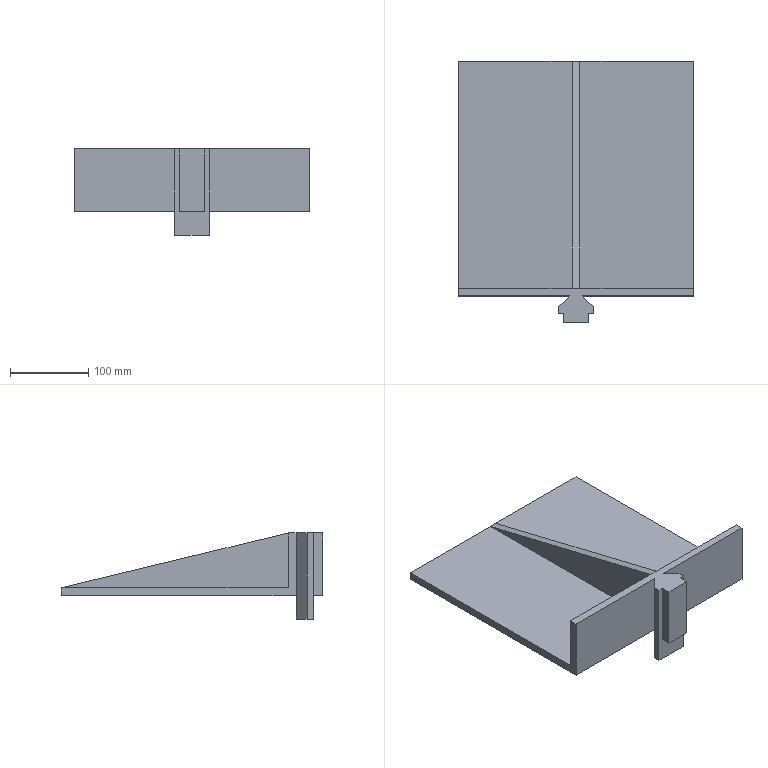Part | STEP file | tuishuban | 1 solid | 25 faces | box 300 x 334 x 110 mm | volume 1327140 mm3 | plane 25